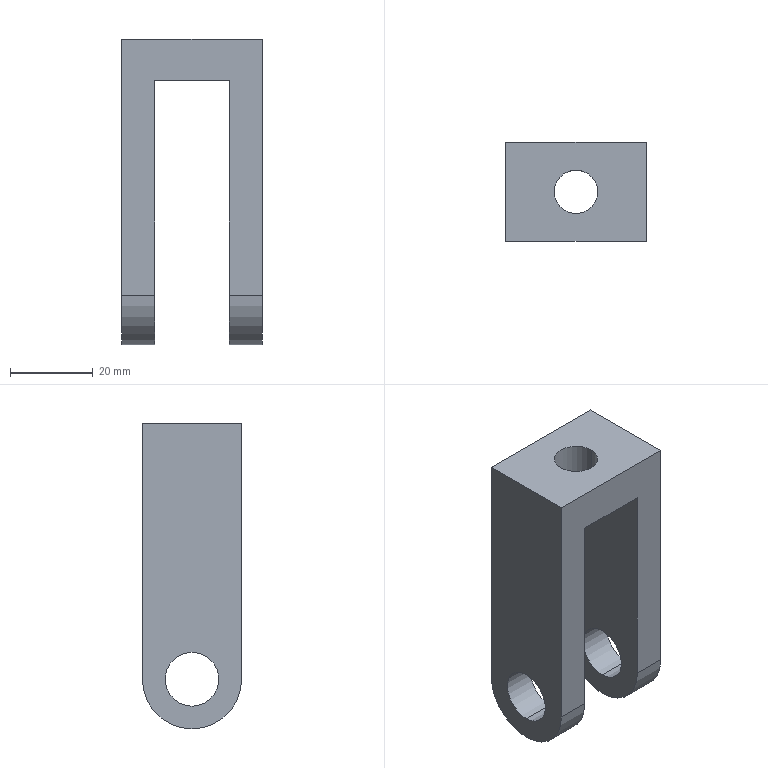Part | SolidWorks | features BaseBody 1 | 1 solid | 16 faces | box 34 x 24 x 74 mm | volume 28757 mm3 | cylinder 8 | plane 8 | commonest cylinder face diameters 13 x4 10.5 x2 24 x2
STEP:
#1=CARTESIAN_POINT('',(861.904,-3537.473,535.578));
#2=VERTEX_POINT('',#1);
#3=CARTESIAN_POINT('',(861.904,-3537.473,548.578));
#4=VERTEX_POINT('',#3);
#5=CARTESIAN_POINT('',(861.904,-3537.473,542.078));
#6=DIRECTION('',(-1.,0.,0.));
#7=DIRECTION('',(0.,0.,-1.));
#8=AXIS2_PLACEMENT_3D('',#5,#6,#7);
#9=CIRCLE('',#8,6.5);
#10=EDGE_CURVE('',#2,#4,#9,.T.);
#11=ORIENTED_EDGE('',*,*,#10,.T.);
#12=CARTESIAN_POINT('',(869.904,-3537.473,548.578));
#13=VERTEX_POINT('',#12);
#14=CARTESIAN_POINT('',(861.904,-3537.473,548.578));
#15=DIRECTION('',(1.,0.,0.));
#16=VECTOR('',#15,1000.);
#17=LINE('',#14,#16);
#18=EDGE_CURVE('',#4,#13,#17,.T.);
#19=ORIENTED_EDGE('',*,*,#18,.T.);
#20=CARTESIAN_POINT('',(869.904,-3537.473,535.578));
#21=VERTEX_POINT('',#20);
#22=CARTESIAN_POINT('',(869.904,-3537.473,542.078));
#23=DIRECTION('',(1.,0.,0.));
#24=DIRECTION('',(0.,0.,-1.));
#25=AXIS2_PLACEMENT_3D('',#22,#23,#24);
#26=CIRCLE('',#25,6.5);
#27=EDGE_CURVE('',#13,#21,#26,.T.);
#28=ORIENTED_EDGE('',*,*,#27,.T.);
#29=CARTESIAN_POINT('',(861.904,-3537.473,535.578));
#30=DIRECTION('',(1.,0.,0.));
#31=VECTOR('',#30,1000.);
#32=LINE('',#29,#31);
#33=EDGE_CURVE('',#2,#21,#32,.T.);
#34=ORIENTED_EDGE('',*,*,#33,.F.);
#35=EDGE_LOOP('',(#11,#19,#28,#34));
#36=FACE_OUTER_BOUND('',#35,.T.);
#37=CARTESIAN_POINT('',(861.904,-3537.473,542.078));
#38=DIRECTION('',(1.,0.,0.));
#39=DIRECTION('',(0.,0.,-1.));
#40=AXIS2_PLACEMENT_3D('',#37,#38,#39);
#41=CYLINDRICAL_SURFACE('',#40,6.5);
#42=ADVANCED_FACE('',(#36),#41,.F.);
#43=CARTESIAN_POINT('',(873.654,-3537.473,594.078));
#44=VERTEX_POINT('',#43);
#45=CARTESIAN_POINT('',(884.154,-3537.473,594.078));
#46=VERTEX_POINT('',#45);
#47=CARTESIAN_POINT('',(878.904,-3537.473,594.078));
#48=DIRECTION('',(0.,0.,1.));
#49=DIRECTION('',(1.,0.,0.));
#50=AXIS2_PLACEMENT_3D('',#47,#48,#49);
#51=CIRCLE('',#50,5.25);
#52=EDGE_CURVE('',#44,#46,#51,.T.);
#53=ORIENTED_EDGE('',*,*,#52,.F.);
#54=CARTESIAN_POINT('',(873.654,-3537.473,604.078));
#55=VERTEX_POINT('',#54);
#56=CARTESIAN_POINT('',(873.654,-3537.473,604.078));
#57=DIRECTION('',(0.,0.,1.));
#58=VECTOR('',#57,1000.);
#59=LINE('',#56,#58);
#60=EDGE_CURVE('',#44,#55,#59,.T.);
#61=ORIENTED_EDGE('',*,*,#60,.T.);
#62=CARTESIAN_POINT('',(884.154,-3537.473,604.078));
#63=VERTEX_POINT('',#62);
#64=CARTESIAN_POINT('',(878.904,-3537.473,604.078));
#65=DIRECTION('',(0.,0.,-1.));
#66=DIRECTION('',(1.,0.,0.));
#67=AXIS2_PLACEMENT_3D('',#64,#65,#66);
#68=CIRCLE('',#67,5.25);
#69=EDGE_CURVE('',#63,#55,#68,.T.);
#70=ORIENTED_EDGE('',*,*,#69,.F.);
#71=CARTESIAN_POINT('',(884.154,-3537.473,604.078));
#72=DIRECTION('',(0.,0.,1.));
#73=VECTOR('',#72,1000.);
#74=LINE('',#71,#73);
#75=EDGE_CURVE('',#46,#63,#74,.T.);
#76=ORIENTED_EDGE('',*,*,#75,.F.);
#77=EDGE_LOOP('',(#53,#61,#70,#76));
#78=FACE_OUTER_BOUND('',#77,.T.);
#79=CARTESIAN_POINT('',(878.904,-3537.473,604.078));
#80=DIRECTION('',(0.,0.,1.));
#81=DIRECTION('',(1.,0.,0.));
#82=AXIS2_PLACEMENT_3D('',#79,#80,#81);
#83=CYLINDRICAL_SURFACE('',#82,5.25);
#84=ADVANCED_FACE('',(#78),#83,.F.);
#85=CARTESIAN_POINT('',(887.904,-3537.473,535.578));
#86=VERTEX_POINT('',#85);
#87=CARTESIAN_POINT('',(887.904,-3537.473,548.578));
#88=VERTEX_POINT('',#87);
#89=CARTESIAN_POINT('',(887.904,-3537.473,542.078));
#90=DIRECTION('',(-1.,0.,0.));
#91=DIRECTION('',(0.,0.,-1.));
#92=AXIS2_PLACEMENT_3D('',#89,#90,#91);
#93=CIRCLE('',#92,6.5);
#94=EDGE_CURVE('',#86,#88,#93,.T.);
#95=ORIENTED_EDGE('',*,*,#94,.T.);
#96=CARTESIAN_POINT('',(895.904,-3537.473,548.578));
#97=VERTEX_POINT('',#96);
#98=CARTESIAN_POINT('',(887.904,-3537.473,548.578));
#99=DIRECTION('',(1.,0.,0.));
#100=VECTOR('',#99,1000.);
#101=LINE('',#98,#100);
#102=EDGE_CURVE('',#88,#97,#101,.T.);
#103=ORIENTED_EDGE('',*,*,#102,.T.);
#104=CARTESIAN_POINT('',(895.904,-3537.473,535.578));
#105=VERTEX_POINT('',#104);
#106=CARTESIAN_POINT('',(895.904,-3537.473,542.078));
#107=DIRECTION('',(-1.,0.,0.));
#108=DIRECTION('',(0.,0.,-1.));
#109=AXIS2_PLACEMENT_3D('',#106,#107,#108);
#110=CIRCLE('',#109,6.5);
#111=EDGE_CURVE('',#105,#97,#110,.T.);
#112=ORIENTED_EDGE('',*,*,#111,.F.);
#113=CARTESIAN_POINT('',(887.904,-3537.473,535.578));
#114=DIRECTION('',(1.,0.,0.));
#115=VECTOR('',#114,1000.);
#116=LINE('',#113,#115);
#117=EDGE_CURVE('',#86,#105,#116,.T.);
#118=ORIENTED_EDGE('',*,*,#117,.F.);
#119=EDGE_LOOP('',(#95,#103,#112,#118));
#120=FACE_OUTER_BOUND('',#119,.T.);
#121=CARTESIAN_POINT('',(887.904,-3537.473,542.078));
#122=DIRECTION('',(1.,0.,0.));
#123=DIRECTION('',(0.,0.,-1.));
#124=AXIS2_PLACEMENT_3D('',#121,#122,#123);
#125=CYLINDRICAL_SURFACE('',#124,6.5);
#126=ADVANCED_FACE('',(#120),#125,.F.);
#127=CARTESIAN_POINT('',(861.904,-3549.473,542.078));
#128=VERTEX_POINT('',#127);
#129=CARTESIAN_POINT('',(861.904,-3525.473,542.078));
#130=VERTEX_POINT('',#129);
#131=CARTESIAN_POINT('',(861.904,-3537.473,542.078));
#132=DIRECTION('',(1.,0.,0.));
#133=DIRECTION('',(0.,1.,0.));
#134=AXIS2_PLACEMENT_3D('',#131,#132,#133);
#135=CIRCLE('',#134,12.);
#136=EDGE_CURVE('',#128,#130,#135,.T.);
#137=ORIENTED_EDGE('',*,*,#136,.F.);
#138=CARTESIAN_POINT('',(861.904,-3549.473,604.078));
#139=VERTEX_POINT('',#138);
#140=CARTESIAN_POINT('',(861.904,-3549.473,599.078));
#141=DIRECTION('',(0.,0.,-1.));
#142=VECTOR('',#141,1000.);
#143=LINE('',#140,#142);
#144=EDGE_CURVE('',#139,#128,#143,.T.);
#145=ORIENTED_EDGE('',*,*,#144,.F.);
#146=CARTESIAN_POINT('',(861.904,-3525.473,604.078));
#147=VERTEX_POINT('',#146);
#148=CARTESIAN_POINT('',(861.904,-3537.473,604.078));
#149=DIRECTION('',(0.,-1.,0.));
#150=VECTOR('',#149,1000.);
#151=LINE('',#148,#150);
#152=EDGE_CURVE('',#147,#139,#151,.T.);
#153=ORIENTED_EDGE('',*,*,#152,.F.);
#154=CARTESIAN_POINT('',(861.904,-3525.473,599.078));
#155=DIRECTION('',(0.,0.,1.));
#156=VECTOR('',#155,1000.);
#157=LINE('',#154,#156);
#158=EDGE_CURVE('',#130,#147,#157,.T.);
#159=ORIENTED_EDGE('',*,*,#158,.F.);
#160=EDGE_LOOP('',(#137,#145,#153,#159));
#161=FACE_OUTER_BOUND('',#160,.T.);
#162=ORIENTED_EDGE('',*,*,#10,.F.);
#163=CARTESIAN_POINT('',(861.904,-3537.473,542.078));
#164=DIRECTION('',(-1.,0.,0.));
#165=DIRECTION('',(0.,0.,-1.));
#166=AXIS2_PLACEMENT_3D('',#163,#164,#165);
#167=CIRCLE('',#166,6.5);
#168=EDGE_CURVE('',#4,#2,#167,.T.);
#169=ORIENTED_EDGE('',*,*,#168,.F.);
#170=EDGE_LOOP('',(#162,#169));
#171=FACE_BOUND('',#170,.T.);
#172=CARTESIAN_POINT('',(861.904,-3537.473,599.078));
#173=DIRECTION('',(1.,0.,0.));
#174=DIRECTION('',(0.,1.,0.));
#175=AXIS2_PLACEMENT_3D('',#172,#173,#174);
#176=PLANE('',#175);
#177=ADVANCED_FACE('',(#161,#171),#176,.F.);
#178=CARTESIAN_POINT('',(869.904,-3525.473,542.078));
#179=VERTEX_POINT('',#178);
#180=CARTESIAN_POINT('',(895.904,-3525.473,542.078));
#181=DIRECTION('',(-1.,0.,0.));
#182=VECTOR('',#181,1000.);
#183=LINE('',#180,#182);
#184=EDGE_CURVE('',#179,#130,#183,.T.);
#185=ORIENTED_EDGE('',*,*,#184,.T.);
#186=ORIENTED_EDGE('',*,*,#158,.T.);
#187=CARTESIAN_POINT('',(895.904,-3525.473,604.078));
#188=VERTEX_POINT('',#187);
#189=CARTESIAN_POINT('',(895.904,-3525.473,604.078));
#190=DIRECTION('',(1.,0.,0.));
#191=VECTOR('',#190,1000.);
#192=LINE('',#189,#191);
#193=EDGE_CURVE('',#147,#188,#192,.T.);
#194=ORIENTED_EDGE('',*,*,#193,.T.);
#195=CARTESIAN_POINT('',(895.904,-3525.473,542.078));
#196=VERTEX_POINT('',#195);
#197=CARTESIAN_POINT('',(895.904,-3525.473,604.078));
#198=DIRECTION('',(0.,0.,-1.));
#199=VECTOR('',#198,1000.);
#200=LINE('',#197,#199);
#201=EDGE_CURVE('',#188,#196,#200,.T.);
#202=ORIENTED_EDGE('',*,*,#201,.T.);
#203=CARTESIAN_POINT('',(887.904,-3525.473,542.078));
#204=VERTEX_POINT('',#203);
#205=CARTESIAN_POINT('',(895.904,-3525.473,542.078));
#206=DIRECTION('',(-1.,0.,0.));
#207=VECTOR('',#206,1000.);
#208=LINE('',#205,#207);
#209=EDGE_CURVE('',#196,#204,#208,.T.);
#210=ORIENTED_EDGE('',*,*,#209,.T.);
#211=CARTESIAN_POINT('',(887.904,-3525.473,594.078));
#212=VERTEX_POINT('',#211);
#213=CARTESIAN_POINT('',(887.904,-3525.473,604.078));
#214=DIRECTION('',(0.,0.,1.));
#215=VECTOR('',#214,1000.);
#216=LINE('',#213,#215);
#217=EDGE_CURVE('',#204,#212,#216,.T.);
#218=ORIENTED_EDGE('',*,*,#217,.T.);
#219=CARTESIAN_POINT('',(869.904,-3525.473,594.078));
#220=VERTEX_POINT('',#219);
#221=CARTESIAN_POINT('',(895.904,-3525.473,594.078));
#222=DIRECTION('',(-1.,0.,0.));
#223=VECTOR('',#222,1000.);
#224=LINE('',#221,#223);
#225=EDGE_CURVE('',#212,#220,#224,.T.);
#226=ORIENTED_EDGE('',*,*,#225,.T.);
#227=CARTESIAN_POINT('',(869.904,-3525.473,604.078));
#228=DIRECTION('',(0.,0.,-1.));
#229=VECTOR('',#228,1000.);
#230=LINE('',#227,#229);
#231=EDGE_CURVE('',#220,#179,#230,.T.);
#232=ORIENTED_EDGE('',*,*,#231,.T.);
#233=EDGE_LOOP('',(#185,#186,#194,#202,#210,#218,#226,#232));
#234=FACE_OUTER_BOUND('',#233,.T.);
#235=CARTESIAN_POINT('',(895.904,-3525.473,604.078));
#236=DIRECTION('',(0.,1.,0.));
#237=DIRECTION('',(0.,0.,1.));
#238=AXIS2_PLACEMENT_3D('',#235,#236,#237);
#239=PLANE('',#238);
#240=ADVANCED_FACE('',(#234),#239,.T.);
#241=CARTESIAN_POINT('',(869.904,-3549.473,542.078));
#242=VERTEX_POINT('',#241);
#243=CARTESIAN_POINT('',(869.904,-3537.473,542.078));
#244=DIRECTION('',(-1.,0.,0.));
#245=DIRECTION('',(0.,1.,0.));
#246=AXIS2_PLACEMENT_3D('',#243,#244,#245);
#247=CIRCLE('',#246,12.);
#248=EDGE_CURVE('',#179,#242,#247,.T.);
#249=ORIENTED_EDGE('',*,*,#248,.T.);
#250=CARTESIAN_POINT('',(869.904,-3549.473,542.078));
#251=DIRECTION('',(-1.,0.,0.));
#252=VECTOR('',#251,1000.);
#253=LINE('',#250,#252);
#254=EDGE_CURVE('',#242,#128,#253,.T.);
#255=ORIENTED_EDGE('',*,*,#254,.T.);
#256=ORIENTED_EDGE('',*,*,#136,.T.);
#257=ORIENTED_EDGE('',*,*,#184,.F.);
#258=EDGE_LOOP('',(#249,#255,#256,#257));
#259=FACE_OUTER_BOUND('',#258,.T.);
#260=CARTESIAN_POINT('',(869.904,-3537.473,542.078));
#261=DIRECTION('',(1.,0.,0.));
#262=DIRECTION('',(0.,1.,0.));
#263=AXIS2_PLACEMENT_3D('',#260,#261,#262);
#264=CYLINDRICAL_SURFACE('',#263,12.);
#265=ADVANCED_FACE('',(#259),#264,.T.);
#266=ORIENTED_EDGE('',*,*,#254,.F.);
#267=CARTESIAN_POINT('',(869.904,-3549.473,594.078));
#268=VERTEX_POINT('',#267);
#269=CARTESIAN_POINT('',(869.904,-3549.473,594.078));
#270=DIRECTION('',(0.,0.,1.));
#271=VECTOR('',#270,1000.);
#272=LINE('',#269,#271);
#273=EDGE_CURVE('',#242,#268,#272,.T.);
#274=ORIENTED_EDGE('',*,*,#273,.T.);
#275=CARTESIAN_POINT('',(887.904,-3549.473,594.078));
#276=VERTEX_POINT('',#275);
#277=CARTESIAN_POINT('',(895.904,-3549.473,594.078));
#278=DIRECTION('',(1.,0.,0.));
#279=VECTOR('',#278,1000.);
#280=LINE('',#277,#279);
#281=EDGE_CURVE('',#268,#276,#280,.T.);
#282=ORIENTED_EDGE('',*,*,#281,.T.);
#283=CARTESIAN_POINT('',(887.904,-3549.473,542.078));
#284=VERTEX_POINT('',#283);
#285=CARTESIAN_POINT('',(887.904,-3549.473,594.078));
#286=DIRECTION('',(0.,0.,-1.));
#287=VECTOR('',#286,1000.);
#288=LINE('',#285,#287);
#289=EDGE_CURVE('',#276,#284,#288,.T.);
#290=ORIENTED_EDGE('',*,*,#289,.T.);
#291=CARTESIAN_POINT('',(895.904,-3549.473,542.078));
#292=VERTEX_POINT('',#291);
#293=CARTESIAN_POINT('',(895.904,-3549.473,542.078));
#294=DIRECTION('',(1.,0.,0.));
#295=VECTOR('',#294,1000.);
#296=LINE('',#293,#295);
#297=EDGE_CURVE('',#284,#292,#296,.T.);
#298=ORIENTED_EDGE('',*,*,#297,.T.);
#299=CARTESIAN_POINT('',(895.904,-3549.473,604.078));
#300=VERTEX_POINT('',#299);
#301=CARTESIAN_POINT('',(895.904,-3549.473,594.078));
#302=DIRECTION('',(0.,0.,1.));
#303=VECTOR('',#302,1000.);
#304=LINE('',#301,#303);
#305=EDGE_CURVE('',#292,#300,#304,.T.);
#306=ORIENTED_EDGE('',*,*,#305,.T.);
#307=CARTESIAN_POINT('',(895.904,-3549.473,604.078));
#308=DIRECTION('',(-1.,0.,0.));
#309=VECTOR('',#308,1000.);
#310=LINE('',#307,#309);
#311=EDGE_CURVE('',#300,#139,#310,.T.);
#312=ORIENTED_EDGE('',*,*,#311,.T.);
#313=ORIENTED_EDGE('',*,*,#144,.T.);
#314=EDGE_LOOP('',(#266,#274,#282,#290,#298,#306,#312,#313));
#315=FACE_OUTER_BOUND('',#314,.T.);
#316=CARTESIAN_POINT('',(895.904,-3549.473,594.078));
#317=DIRECTION('',(0.,-1.,0.));
#318=DIRECTION('',(1.,0.,0.));
#319=AXIS2_PLACEMENT_3D('',#316,#317,#318);
#320=PLANE('',#319);
#321=ADVANCED_FACE('',(#315),#320,.T.);
#322=ORIENTED_EDGE('',*,*,#193,.F.);
#323=ORIENTED_EDGE('',*,*,#152,.T.);
#324=ORIENTED_EDGE('',*,*,#311,.F.);
#325=CARTESIAN_POINT('',(895.904,-3549.473,604.078));
#326=DIRECTION('',(0.,1.,0.));
#327=VECTOR('',#326,1000.);
#328=LINE('',#325,#327);
#329=EDGE_CURVE('',#300,#188,#328,.T.);
#330=ORIENTED_EDGE('',*,*,#329,.T.);
#331=EDGE_LOOP('',(#322,#323,#324,#330));
#332=FACE_OUTER_BOUND('',#331,.T.);
#333=ORIENTED_EDGE('',*,*,#69,.T.);
#334=CARTESIAN_POINT('',(878.904,-3537.473,604.078));
#335=DIRECTION('',(0.,0.,-1.));
#336=DIRECTION('',(1.,0.,0.));
#337=AXIS2_PLACEMENT_3D('',#334,#335,#336);
#338=CIRCLE('',#337,5.25);
#339=EDGE_CURVE('',#55,#63,#338,.T.);
#340=ORIENTED_EDGE('',*,*,#339,.T.);
#341=EDGE_LOOP('',(#333,#340));
#342=FACE_BOUND('',#341,.T.);
#343=CARTESIAN_POINT('',(895.904,-3549.473,604.078));
#344=DIRECTION('',(0.,0.,1.));
#345=DIRECTION('',(1.,0.,0.));
#346=AXIS2_PLACEMENT_3D('',#343,#344,#345);
#347=PLANE('',#346);
#348=ADVANCED_FACE('',(#332,#342),#347,.T.);
#349=ORIENTED_EDGE('',*,*,#18,.F.);
#350=ORIENTED_EDGE('',*,*,#168,.T.);
#351=ORIENTED_EDGE('',*,*,#33,.T.);
#352=CARTESIAN_POINT('',(869.904,-3537.473,542.078));
#353=DIRECTION('',(1.,0.,0.));
#354=DIRECTION('',(0.,0.,-1.));
#355=AXIS2_PLACEMENT_3D('',#352,#353,#354);
#356=CIRCLE('',#355,6.5);
#357=EDGE_CURVE('',#21,#13,#356,.T.);
#358=ORIENTED_EDGE('',*,*,#357,.T.);
#359=EDGE_LOOP('',(#349,#350,#351,#358));
#360=FACE_OUTER_BOUND('',#359,.T.);
#361=CARTESIAN_POINT('',(861.904,-3537.473,542.078));
#362=DIRECTION('',(1.,0.,0.));
#363=DIRECTION('',(0.,0.,-1.));
#364=AXIS2_PLACEMENT_3D('',#361,#362,#363);
#365=CYLINDRICAL_SURFACE('',#364,6.5);
#366=ADVANCED_FACE('',(#360),#365,.F.);
#367=ORIENTED_EDGE('',*,*,#357,.F.);
#368=ORIENTED_EDGE('',*,*,#27,.F.);
#369=EDGE_LOOP('',(#367,#368));
#370=FACE_BOUND('',#369,.T.);
#371=ORIENTED_EDGE('',*,*,#248,.F.);
#372=ORIENTED_EDGE('',*,*,#231,.F.);
#373=CARTESIAN_POINT('',(869.904,-3537.473,594.078));
#374=DIRECTION('',(0.,-1.,0.));
#375=VECTOR('',#374,1000.);
#376=LINE('',#373,#375);
#377=EDGE_CURVE('',#220,#268,#376,.T.);
#378=ORIENTED_EDGE('',*,*,#377,.T.);
#379=ORIENTED_EDGE('',*,*,#273,.F.);
#380=EDGE_LOOP('',(#371,#372,#378,#379));
#381=FACE_OUTER_BOUND('',#380,.T.);
#382=CARTESIAN_POINT('',(869.904,-3537.473,569.274));
#383=DIRECTION('',(1.,0.,0.));
#384=DIRECTION('',(0.,1.,0.));
#385=AXIS2_PLACEMENT_3D('',#382,#383,#384);
#386=PLANE('',#385);
#387=ADVANCED_FACE('',(#370,#381),#386,.T.);
#388=ORIENTED_EDGE('',*,*,#377,.F.);
#389=ORIENTED_EDGE('',*,*,#225,.F.);
#390=CARTESIAN_POINT('',(887.904,-3525.473,594.078));
#391=DIRECTION('',(0.,-1.,0.));
#392=VECTOR('',#391,1000.);
#393=LINE('',#390,#392);
#394=EDGE_CURVE('',#212,#276,#393,.T.);
#395=ORIENTED_EDGE('',*,*,#394,.T.);
#396=ORIENTED_EDGE('',*,*,#281,.F.);
#397=EDGE_LOOP('',(#388,#389,#395,#396));
#398=FACE_OUTER_BOUND('',#397,.T.);
#399=CARTESIAN_POINT('',(878.904,-3537.473,594.078));
#400=DIRECTION('',(0.,0.,1.));
#401=DIRECTION('',(1.,0.,0.));
#402=AXIS2_PLACEMENT_3D('',#399,#400,#401);
#403=CIRCLE('',#402,5.25);
#404=EDGE_CURVE('',#46,#44,#403,.T.);
#405=ORIENTED_EDGE('',*,*,#404,.T.);
#406=ORIENTED_EDGE('',*,*,#52,.T.);
#407=EDGE_LOOP('',(#405,#406));
#408=FACE_BOUND('',#407,.T.);
#409=CARTESIAN_POINT('',(895.904,-3525.473,594.078));
#410=DIRECTION('',(0.,0.,-1.));
#411=DIRECTION('',(-1.,0.,0.));
#412=AXIS2_PLACEMENT_3D('',#409,#410,#411);
#413=PLANE('',#412);
#414=ADVANCED_FACE('',(#398,#408),#413,.T.);
#415=ORIENTED_EDGE('',*,*,#94,.F.);
#416=CARTESIAN_POINT('',(887.904,-3537.473,542.078));
#417=DIRECTION('',(-1.,0.,0.));
#418=DIRECTION('',(0.,0.,-1.));
#419=AXIS2_PLACEMENT_3D('',#416,#417,#418);
#420=CIRCLE('',#419,6.5);
#421=EDGE_CURVE('',#88,#86,#420,.T.);
#422=ORIENTED_EDGE('',*,*,#421,.F.);
#423=EDGE_LOOP('',(#415,#422));
#424=FACE_BOUND('',#423,.T.);
#425=ORIENTED_EDGE('',*,*,#217,.F.);
#426=CARTESIAN_POINT('',(887.904,-3537.473,542.078));
#427=DIRECTION('',(1.,0.,0.));
#428=DIRECTION('',(0.,1.,0.));
#429=AXIS2_PLACEMENT_3D('',#426,#427,#428);
#430=CIRCLE('',#429,12.);
#431=EDGE_CURVE('',#284,#204,#430,.T.);
#432=ORIENTED_EDGE('',*,*,#431,.F.);
#433=ORIENTED_EDGE('',*,*,#289,.F.);
#434=ORIENTED_EDGE('',*,*,#394,.F.);
#435=EDGE_LOOP('',(#425,#432,#433,#434));
#436=FACE_OUTER_BOUND('',#435,.T.);
#437=CARTESIAN_POINT('',(887.904,-3537.473,569.274));
#438=DIRECTION('',(1.,0.,0.));
#439=DIRECTION('',(0.,1.,0.));
#440=AXIS2_PLACEMENT_3D('',#437,#438,#439);
#441=PLANE('',#440);
#442=ADVANCED_FACE('',(#424,#436),#441,.F.);
#443=CARTESIAN_POINT('',(895.904,-3537.473,542.078));
#444=DIRECTION('',(-1.,0.,0.));
#445=DIRECTION('',(0.,1.,0.));
#446=AXIS2_PLACEMENT_3D('',#443,#444,#445);
#447=CIRCLE('',#446,12.);
#448=EDGE_CURVE('',#196,#292,#447,.T.);
#449=ORIENTED_EDGE('',*,*,#448,.T.);
#450=ORIENTED_EDGE('',*,*,#297,.F.);
#451=ORIENTED_EDGE('',*,*,#431,.T.);
#452=ORIENTED_EDGE('',*,*,#209,.F.);
#453=EDGE_LOOP('',(#449,#450,#451,#452));
#454=FACE_OUTER_BOUND('',#453,.T.);
#455=CARTESIAN_POINT('',(895.904,-3537.473,542.078));
#456=DIRECTION('',(1.,0.,0.));
#457=DIRECTION('',(0.,1.,0.));
#458=AXIS2_PLACEMENT_3D('',#455,#456,#457);
#459=CYLINDRICAL_SURFACE('',#458,12.);
#460=ADVANCED_FACE('',(#454),#459,.T.);
#461=ORIENTED_EDGE('',*,*,#448,.F.);
#462=ORIENTED_EDGE('',*,*,#201,.F.);
#463=ORIENTED_EDGE('',*,*,#329,.F.);
#464=ORIENTED_EDGE('',*,*,#305,.F.);
#465=EDGE_LOOP('',(#461,#462,#463,#464));
#466=FACE_OUTER_BOUND('',#465,.T.);
#467=ORIENTED_EDGE('',*,*,#111,.T.);
#468=CARTESIAN_POINT('',(895.904,-3537.473,542.078));
#469=DIRECTION('',(-1.,0.,0.));
#470=DIRECTION('',(0.,0.,-1.));
#471=AXIS2_PLACEMENT_3D('',#468,#469,#470);
#472=CIRCLE('',#471,6.5);
#473=EDGE_CURVE('',#97,#105,#472,.T.);
#474=ORIENTED_EDGE('',*,*,#473,.T.);
#475=EDGE_LOOP('',(#467,#474));
#476=FACE_BOUND('',#475,.T.);
#477=CARTESIAN_POINT('',(895.904,-3537.473,599.078));
#478=DIRECTION('',(1.,0.,0.));
#479=DIRECTION('',(0.,1.,0.));
#480=AXIS2_PLACEMENT_3D('',#477,#478,#479);
#481=PLANE('',#480);
#482=ADVANCED_FACE('',(#466,#476),#481,.T.);
#483=ORIENTED_EDGE('',*,*,#60,.F.);
#484=ORIENTED_EDGE('',*,*,#404,.F.);
#485=ORIENTED_EDGE('',*,*,#75,.T.);
#486=ORIENTED_EDGE('',*,*,#339,.F.);
#487=EDGE_LOOP('',(#483,#484,#485,#486));
#488=FACE_OUTER_BOUND('',#487,.T.);
#489=CARTESIAN_POINT('',(878.904,-3537.473,604.078));
#490=DIRECTION('',(0.,0.,1.));
#491=DIRECTION('',(1.,0.,0.));
#492=AXIS2_PLACEMENT_3D('',#489,#490,#491);
#493=CYLINDRICAL_SURFACE('',#492,5.25);
#494=ADVANCED_FACE('',(#488),#493,.F.);
#495=ORIENTED_EDGE('',*,*,#102,.F.);
#496=ORIENTED_EDGE('',*,*,#421,.T.);
#497=ORIENTED_EDGE('',*,*,#117,.T.);
#498=ORIENTED_EDGE('',*,*,#473,.F.);
#499=EDGE_LOOP('',(#495,#496,#497,#498));
#500=FACE_OUTER_BOUND('',#499,.T.);
#501=CARTESIAN_POINT('',(887.904,-3537.473,542.078));
#502=DIRECTION('',(1.,0.,0.));
#503=DIRECTION('',(0.,0.,-1.));
#504=AXIS2_PLACEMENT_3D('',#501,#502,#503);
#505=CYLINDRICAL_SURFACE('',#504,6.5);
#506=ADVANCED_FACE('',(#500),#505,.F.);
#507=CLOSED_SHELL('',(#42,#84,#126,#177,#240,#265,#321,#348,#366,#387,#414,#442,#460,#482,#494,#506));
#508=MANIFOLD_SOLID_BREP('',#507);
#509=CARTESIAN_POINT('',(0.,0.,0.));
#510=DIRECTION('',(0.,0.,1.));
#511=DIRECTION('',(1.,0.,0.));
#512=AXIS2_PLACEMENT_3D('',#509,#510,#511);
#513=(LENGTH_UNIT()NAMED_UNIT(*)SI_UNIT(.MILLI.,.METRE.));
#514=UNCERTAINTY_MEASURE_WITH_UNIT(LENGTH_MEASURE(0.00001),#513,'','');
#515=(NAMED_UNIT(*)PLANE_ANGLE_UNIT()SI_UNIT($,.RADIAN.));
#516=(NAMED_UNIT(*)SI_UNIT($,.STERADIAN.)SOLID_ANGLE_UNIT());
#517=(GEOMETRIC_REPRESENTATION_CONTEXT(3)GLOBAL_UNCERTAINTY_ASSIGNED_CONTEXT((#514))GLOBAL_UNIT_ASSIGNED_CONTEXT((#513,#515,#516))REPRESENTATION_CONTEXT('',''));
#518=ADVANCED_BREP_SHAPE_REPRESENTATION('',(#508,#512),#517);